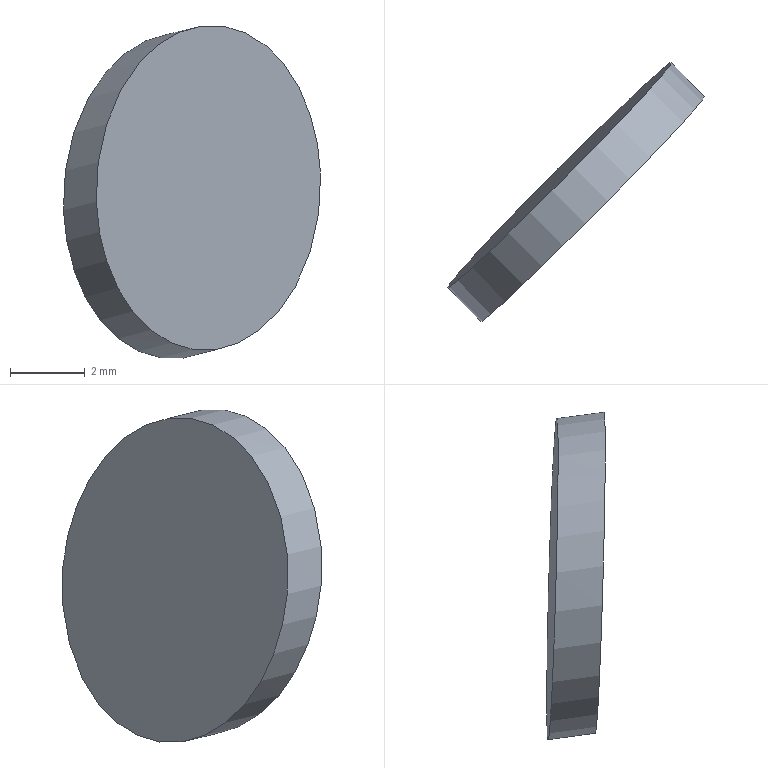Part | STEP file | gslz 2016.10.28-13_id1062_x_t | 1 solid | 3 faces | box 6.872 x 6.937 x 8.903 mm | volume 72.493 mm3 | spline 2 | cylinder 1 | commonest cylinder face diameters 8.5 x1
STEP:
#1=CARTESIAN_POINT('',(0.,0.,0.));
#2=DIRECTION('',(0.,0.,1.));
#3=DIRECTION('',(1.,0.,0.));
#4=AXIS2_PLACEMENT_3D('',#1,#2,#3);
#5=CARTESIAN_POINT('',(99.595,227.749,-30.31));
#6=VERTEX_POINT('',#5);
#7=CARTESIAN_POINT('',(93.608,221.761,-31.051));
#8=VERTEX_POINT('',#7);
#9=CARTESIAN_POINT('',(99.595,227.749,-30.31));
#10=CARTESIAN_POINT('',(99.637,227.846,-31.43));
#11=CARTESIAN_POINT('',(99.364,227.628,-32.586));
#12=CARTESIAN_POINT('',(98.322,226.666,-34.332));
#13=CARTESIAN_POINT('',(97.554,225.922,-34.908));
#14=CARTESIAN_POINT('',(95.969,224.337,-35.104));
#15=CARTESIAN_POINT('',(95.167,223.511,-34.722));
#16=CARTESIAN_POINT('',(94.005,222.269,-33.249));
#17=CARTESIAN_POINT('',(93.649,221.858,-32.171));
#18=CARTESIAN_POINT('',(93.608,221.761,-31.051));
#19=B_SPLINE_CURVE_WITH_KNOTS('',3,(#9,#10,#11,#12,#13,#14,#15,#16,#17,#18),.UNSPECIFIED.,.F.,.F.,(4,2,2,2,4),(0.,0.25,0.5,0.75,1.),.UNSPECIFIED.);
#20=CARTESIAN_POINT('',(82.862,211.656,-45.368));
#21=CARTESIAN_POINT('',(82.657,211.178,-39.851));
#22=CARTESIAN_POINT('',(82.452,210.7,-34.333));
#23=CARTESIAN_POINT('',(82.248,210.222,-28.816));
#24=CARTESIAN_POINT('',(82.043,209.744,-23.299));
#25=CARTESIAN_POINT('',(81.839,209.265,-17.782));
#26=CARTESIAN_POINT('',(88.082,216.876,-44.722));
#27=CARTESIAN_POINT('',(87.877,216.398,-39.205));
#28=CARTESIAN_POINT('',(87.673,215.92,-33.688));
#29=CARTESIAN_POINT('',(87.468,215.442,-28.17));
#30=CARTESIAN_POINT('',(87.264,214.964,-22.653));
#31=CARTESIAN_POINT('',(87.059,214.486,-17.136));
#32=CARTESIAN_POINT('',(93.302,222.096,-44.076));
#33=CARTESIAN_POINT('',(93.098,221.618,-38.559));
#34=CARTESIAN_POINT('',(92.893,221.14,-33.042));
#35=CARTESIAN_POINT('',(92.688,220.662,-27.524));
#36=CARTESIAN_POINT('',(92.484,220.184,-22.007));
#37=CARTESIAN_POINT('',(92.279,219.706,-16.49));
#38=CARTESIAN_POINT('',(98.522,227.317,-43.43));
#39=CARTESIAN_POINT('',(98.318,226.839,-37.913));
#40=CARTESIAN_POINT('',(98.113,226.361,-32.396));
#41=CARTESIAN_POINT('',(97.909,225.882,-26.879));
#42=CARTESIAN_POINT('',(97.704,225.404,-21.361));
#43=CARTESIAN_POINT('',(97.5,224.926,-15.844));
#44=CARTESIAN_POINT('',(103.743,232.537,-42.784));
#45=CARTESIAN_POINT('',(103.538,232.059,-37.267));
#46=CARTESIAN_POINT('',(103.334,231.581,-31.75));
#47=CARTESIAN_POINT('',(103.129,231.103,-26.233));
#48=CARTESIAN_POINT('',(102.924,230.625,-20.715));
#49=CARTESIAN_POINT('',(102.72,230.147,-15.198));
#50=CARTESIAN_POINT('',(108.963,237.757,-42.139));
#51=CARTESIAN_POINT('',(108.758,237.279,-36.621));
#52=CARTESIAN_POINT('',(108.554,236.801,-31.104));
#53=CARTESIAN_POINT('',(108.349,236.323,-25.587));
#54=CARTESIAN_POINT('',(108.145,235.845,-20.07));
#55=CARTESIAN_POINT('',(107.94,235.367,-14.552));
#56=B_SPLINE_SURFACE_WITH_KNOTS('',5,5,((#20,#21,#22,#23,#24,#25),(#26,#27,#28,#29,#30,#31),(#32,#33,#34,#35,#36,#37),(#38,#39,#40,#41,#42,#43),(#44,#45,#46,#47,#48,#49),(#50,#51,#52,#53,#54,#55)),.UNSPECIFIED.,.F.,.F.,.F.,(6,6),(6,6),(0.,1.),(0.,1.),.PIECEWISE_BEZIER_KNOTS.);
#57=CARTESIAN_POINT('',(0.6595,0.4687));
#58=CARTESIAN_POINT('',(0.6595,0.4613));
#59=CARTESIAN_POINT('',(0.6587,0.4465));
#60=CARTESIAN_POINT('',(0.6552,0.4248));
#61=CARTESIAN_POINT('',(0.6496,0.4039));
#62=CARTESIAN_POINT('',(0.6418,0.3843));
#63=CARTESIAN_POINT('',(0.6322,0.3663));
#64=CARTESIAN_POINT('',(0.6206,0.3503));
#65=CARTESIAN_POINT('',(0.6074,0.3368));
#66=CARTESIAN_POINT('',(0.593,0.326));
#67=CARTESIAN_POINT('',(0.5775,0.318));
#68=CARTESIAN_POINT('',(0.5613,0.313));
#69=CARTESIAN_POINT('',(0.5448,0.3113));
#70=CARTESIAN_POINT('',(0.5282,0.313));
#71=CARTESIAN_POINT('',(0.5121,0.318));
#72=CARTESIAN_POINT('',(0.4966,0.326));
#73=CARTESIAN_POINT('',(0.4821,0.3368));
#74=CARTESIAN_POINT('',(0.4689,0.3503));
#75=CARTESIAN_POINT('',(0.4574,0.3663));
#76=CARTESIAN_POINT('',(0.4477,0.3843));
#77=CARTESIAN_POINT('',(0.44,0.4039));
#78=CARTESIAN_POINT('',(0.4343,0.4248));
#79=CARTESIAN_POINT('',(0.4309,0.4465));
#80=CARTESIAN_POINT('',(0.4301,0.4613));
#81=CARTESIAN_POINT('',(0.4301,0.4687));
#82=B_SPLINE_CURVE_WITH_KNOTS('',3,(#57,#58,#59,#60,#61,#62,#63,#64,#65,#66,#67,#68,#69,#70,#71,#72,#73,#74,#75,#76,#77,#78,#79,#80,#81),.UNSPECIFIED.,.F.,.F.,(4,1,1,1,1,1,1,1,1,1,1,1,1,1,1,1,1,1,1,1,1,1,4),(0.,0.04545,0.09091,0.1364,0.1818,0.2273,0.2727,0.3182,0.3636,0.4091,0.4545,0.5,0.5455,0.5909,0.6364,0.6818,0.7273,0.7727,0.8182,0.8636,0.9091,0.9545,1.),.QUASI_UNIFORM_KNOTS.);
#83=(GEOMETRIC_REPRESENTATION_CONTEXT(2)PARAMETRIC_REPRESENTATION_CONTEXT()REPRESENTATION_CONTEXT('',''));
#84=DEFINITIONAL_REPRESENTATION('',(#82),#83);
#85=PCURVE('',#56,#84);
#86=CARTESIAN_POINT('',(96.602,224.755,-30.68));
#87=DIRECTION('',(0.6857,-0.7071,0.173));
#88=DIRECTION('',(-0.1835,0.06209,0.9811));
#89=AXIS2_PLACEMENT_3D('',#86,#87,#88);
#90=CYLINDRICAL_SURFACE('',#89,4.25);
#91=CARTESIAN_POINT('',(4.712,0.));
#92=CARTESIAN_POINT('',(4.665,-0.04253));
#93=CARTESIAN_POINT('',(4.571,-0.1275));
#94=CARTESIAN_POINT('',(4.43,-0.2526));
#95=CARTESIAN_POINT('',(4.288,-0.3729));
#96=CARTESIAN_POINT('',(4.146,-0.486));
#97=CARTESIAN_POINT('',(4.004,-0.5898));
#98=CARTESIAN_POINT('',(3.861,-0.6818));
#99=CARTESIAN_POINT('',(3.718,-0.7595));
#100=CARTESIAN_POINT('',(3.574,-0.822));
#101=CARTESIAN_POINT('',(3.43,-0.8682));
#102=CARTESIAN_POINT('',(3.286,-0.8968));
#103=CARTESIAN_POINT('',(3.142,-0.9067));
#104=CARTESIAN_POINT('',(2.997,-0.8968));
#105=CARTESIAN_POINT('',(2.853,-0.8682));
#106=CARTESIAN_POINT('',(2.709,-0.822));
#107=CARTESIAN_POINT('',(2.565,-0.7595));
#108=CARTESIAN_POINT('',(2.422,-0.6818));
#109=CARTESIAN_POINT('',(2.279,-0.5898));
#110=CARTESIAN_POINT('',(2.137,-0.486));
#111=CARTESIAN_POINT('',(1.995,-0.3729));
#112=CARTESIAN_POINT('',(1.853,-0.2526));
#113=CARTESIAN_POINT('',(1.712,-0.1275));
#114=CARTESIAN_POINT('',(1.618,-0.04253));
#115=CARTESIAN_POINT('',(1.571,0.));
#116=B_SPLINE_CURVE_WITH_KNOTS('',3,(#91,#92,#93,#94,#95,#96,#97,#98,#99,#100,#101,#102,#103,#104,#105,#106,#107,#108,#109,#110,#111,#112,#113,#114,#115),.UNSPECIFIED.,.F.,.F.,(4,1,1,1,1,1,1,1,1,1,1,1,1,1,1,1,1,1,1,1,1,1,4),(0.,0.04545,0.09091,0.1364,0.1818,0.2273,0.2727,0.3182,0.3636,0.4091,0.4545,0.5,0.5455,0.5909,0.6364,0.6818,0.7273,0.7727,0.8182,0.8636,0.9091,0.9545,1.),.QUASI_UNIFORM_KNOTS.);
#117=(GEOMETRIC_REPRESENTATION_CONTEXT(2)PARAMETRIC_REPRESENTATION_CONTEXT()REPRESENTATION_CONTEXT('',''));
#118=DEFINITIONAL_REPRESENTATION('',(#116),#117);
#119=PCURVE('',#90,#118);
#120=SURFACE_CURVE('',#19,(#85,#119),.PCURVE_S1.);
#121=EDGE_CURVE('',#6,#8,#120,.T.);
#122=ORIENTED_EDGE('',*,*,#121,.F.);
#123=CARTESIAN_POINT('',(93.608,221.761,-31.051));
#124=CARTESIAN_POINT('',(93.566,221.664,-29.931));
#125=CARTESIAN_POINT('',(93.839,221.881,-28.775));
#126=CARTESIAN_POINT('',(94.881,222.844,-27.029));
#127=CARTESIAN_POINT('',(95.649,223.588,-26.453));
#128=CARTESIAN_POINT('',(97.234,225.173,-26.256));
#129=CARTESIAN_POINT('',(98.036,225.999,-26.638));
#130=CARTESIAN_POINT('',(99.198,227.241,-28.112));
#131=CARTESIAN_POINT('',(99.554,227.652,-29.19));
#132=CARTESIAN_POINT('',(99.595,227.749,-30.31));
#133=B_SPLINE_CURVE_WITH_KNOTS('',3,(#123,#124,#125,#126,#127,#128,#129,#130,#131,#132),.UNSPECIFIED.,.F.,.F.,(4,2,2,2,4),(0.,0.25,0.5,0.75,1.),.UNSPECIFIED.);
#134=CARTESIAN_POINT('',(0.4301,0.4687));
#135=CARTESIAN_POINT('',(0.4301,0.476));
#136=CARTESIAN_POINT('',(0.4309,0.4908));
#137=CARTESIAN_POINT('',(0.4343,0.5125));
#138=CARTESIAN_POINT('',(0.44,0.5334));
#139=CARTESIAN_POINT('',(0.4477,0.553));
#140=CARTESIAN_POINT('',(0.4574,0.571));
#141=CARTESIAN_POINT('',(0.4689,0.587));
#142=CARTESIAN_POINT('',(0.4821,0.6005));
#143=CARTESIAN_POINT('',(0.4966,0.6113));
#144=CARTESIAN_POINT('',(0.5121,0.6193));
#145=CARTESIAN_POINT('',(0.5282,0.6243));
#146=CARTESIAN_POINT('',(0.5448,0.626));
#147=CARTESIAN_POINT('',(0.5613,0.6243));
#148=CARTESIAN_POINT('',(0.5775,0.6193));
#149=CARTESIAN_POINT('',(0.593,0.6113));
#150=CARTESIAN_POINT('',(0.6074,0.6005));
#151=CARTESIAN_POINT('',(0.6206,0.587));
#152=CARTESIAN_POINT('',(0.6322,0.571));
#153=CARTESIAN_POINT('',(0.6418,0.553));
#154=CARTESIAN_POINT('',(0.6496,0.5334));
#155=CARTESIAN_POINT('',(0.6552,0.5125));
#156=CARTESIAN_POINT('',(0.6587,0.4908));
#157=CARTESIAN_POINT('',(0.6595,0.476));
#158=CARTESIAN_POINT('',(0.6595,0.4687));
#159=B_SPLINE_CURVE_WITH_KNOTS('',3,(#134,#135,#136,#137,#138,#139,#140,#141,#142,#143,#144,#145,#146,#147,#148,#149,#150,#151,#152,#153,#154,#155,#156,#157,#158),.UNSPECIFIED.,.F.,.F.,(4,1,1,1,1,1,1,1,1,1,1,1,1,1,1,1,1,1,1,1,1,1,4),(0.,0.04545,0.09091,0.1364,0.1818,0.2273,0.2727,0.3182,0.3636,0.4091,0.4545,0.5,0.5455,0.5909,0.6364,0.6818,0.7273,0.7727,0.8182,0.8636,0.9091,0.9545,1.),.QUASI_UNIFORM_KNOTS.);
#160=(GEOMETRIC_REPRESENTATION_CONTEXT(2)PARAMETRIC_REPRESENTATION_CONTEXT()REPRESENTATION_CONTEXT('',''));
#161=DEFINITIONAL_REPRESENTATION('',(#159),#160);
#162=PCURVE('',#56,#161);
#163=CARTESIAN_POINT('',(7.854,0.));
#164=CARTESIAN_POINT('',(7.807,0.04253));
#165=CARTESIAN_POINT('',(7.713,0.1275));
#166=CARTESIAN_POINT('',(7.571,0.2526));
#167=CARTESIAN_POINT('',(7.43,0.3729));
#168=CARTESIAN_POINT('',(7.288,0.486));
#169=CARTESIAN_POINT('',(7.145,0.5898));
#170=CARTESIAN_POINT('',(7.003,0.6818));
#171=CARTESIAN_POINT('',(6.86,0.7595));
#172=CARTESIAN_POINT('',(6.716,0.822));
#173=CARTESIAN_POINT('',(6.572,0.8682));
#174=CARTESIAN_POINT('',(6.427,0.8968));
#175=CARTESIAN_POINT('',(6.283,0.9067));
#176=CARTESIAN_POINT('',(6.139,0.8968));
#177=CARTESIAN_POINT('',(5.995,0.8682));
#178=CARTESIAN_POINT('',(5.851,0.822));
#179=CARTESIAN_POINT('',(5.707,0.7595));
#180=CARTESIAN_POINT('',(5.564,0.6818));
#181=CARTESIAN_POINT('',(5.421,0.5898));
#182=CARTESIAN_POINT('',(5.279,0.486));
#183=CARTESIAN_POINT('',(5.137,0.3729));
#184=CARTESIAN_POINT('',(4.995,0.2526));
#185=CARTESIAN_POINT('',(4.854,0.1275));
#186=CARTESIAN_POINT('',(4.759,0.04253));
#187=CARTESIAN_POINT('',(4.712,0.));
#188=B_SPLINE_CURVE_WITH_KNOTS('',3,(#163,#164,#165,#166,#167,#168,#169,#170,#171,#172,#173,#174,#175,#176,#177,#178,#179,#180,#181,#182,#183,#184,#185,#186,#187),.UNSPECIFIED.,.F.,.F.,(4,1,1,1,1,1,1,1,1,1,1,1,1,1,1,1,1,1,1,1,1,1,4),(0.,0.04545,0.09091,0.1364,0.1818,0.2273,0.2727,0.3182,0.3636,0.4091,0.4545,0.5,0.5455,0.5909,0.6364,0.6818,0.7273,0.7727,0.8182,0.8636,0.9091,0.9545,1.),.QUASI_UNIFORM_KNOTS.);
#189=(GEOMETRIC_REPRESENTATION_CONTEXT(2)PARAMETRIC_REPRESENTATION_CONTEXT()REPRESENTATION_CONTEXT('',''));
#190=DEFINITIONAL_REPRESENTATION('',(#188),#189);
#191=PCURVE('',#90,#190);
#192=SURFACE_CURVE('',#133,(#162,#191),.PCURVE_S1.);
#193=EDGE_CURVE('',#8,#6,#192,.T.);
#194=ORIENTED_EDGE('',*,*,#193,.F.);
#195=EDGE_LOOP('',(#122,#194));
#196=FACE_BOUND('',#195,.F.);
#197=ADVANCED_FACE('',(#196),#56,.F.);
#198=ORIENTED_EDGE('',*,*,#193,.F.);
#199=CARTESIAN_POINT('',(94.484,220.858,-30.83));
#200=VERTEX_POINT('',#199);
#201=CARTESIAN_POINT('',(93.608,221.761,-31.051));
#202=CARTESIAN_POINT('',(94.484,220.858,-30.83));
#203=B_SPLINE_CURVE_WITH_KNOTS('',1,(#201,#202),.UNSPECIFIED.,.F.,.F.,(2,2),(0.,1.278),.PIECEWISE_BEZIER_KNOTS.);
#204=CARTESIAN_POINT('',(7.854,0.));
#205=DIRECTION('',(0.,1.));
#206=VECTOR('',#205,1.);
#207=LINE('',#204,#206);
#208=(GEOMETRIC_REPRESENTATION_CONTEXT(2)PARAMETRIC_REPRESENTATION_CONTEXT()REPRESENTATION_CONTEXT('',''));
#209=DEFINITIONAL_REPRESENTATION('',(#207),#208);
#210=PCURVE('',#90,#209);
#211=CARTESIAN_POINT('',(1.571,0.));
#212=DIRECTION('',(0.,1.));
#213=VECTOR('',#212,1.);
#214=LINE('',#211,#213);
#215=(GEOMETRIC_REPRESENTATION_CONTEXT(2)PARAMETRIC_REPRESENTATION_CONTEXT()REPRESENTATION_CONTEXT('',''));
#216=DEFINITIONAL_REPRESENTATION('',(#214),#215);
#217=PCURVE('',#90,#216);
#218=SEAM_CURVE('',#203,(#210,#217),.PCURVE_S1.);
#219=EDGE_CURVE('',#8,#200,#218,.T.);
#220=ORIENTED_EDGE('',*,*,#219,.T.);
#221=CARTESIAN_POINT('',(100.472,226.845,-30.089));
#222=VERTEX_POINT('',#221);
#223=CARTESIAN_POINT('',(94.484,220.858,-30.83));
#224=CARTESIAN_POINT('',(94.442,220.76,-29.707));
#225=CARTESIAN_POINT('',(94.714,220.977,-28.556));
#226=CARTESIAN_POINT('',(95.759,221.942,-26.805));
#227=CARTESIAN_POINT('',(96.525,222.684,-26.232));
#228=CARTESIAN_POINT('',(98.107,224.266,-26.035));
#229=CARTESIAN_POINT('',(98.908,225.091,-26.412));
#230=CARTESIAN_POINT('',(100.078,226.341,-27.895));
#231=CARTESIAN_POINT('',(100.43,226.748,-28.971));
#232=CARTESIAN_POINT('',(100.472,226.845,-30.089));
#233=B_SPLINE_CURVE_WITH_KNOTS('',3,(#223,#224,#225,#226,#227,#228,#229,#230,#231,#232),.UNSPECIFIED.,.F.,.F.,(4,2,2,2,4),(0.,0.25,0.5,0.75,1.),.UNSPECIFIED.);
#234=CARTESIAN_POINT('',(7.854,1.278));
#235=CARTESIAN_POINT('',(7.807,1.321));
#236=CARTESIAN_POINT('',(7.713,1.406));
#237=CARTESIAN_POINT('',(7.571,1.531));
#238=CARTESIAN_POINT('',(7.43,1.651));
#239=CARTESIAN_POINT('',(7.288,1.764));
#240=CARTESIAN_POINT('',(7.146,1.868));
#241=CARTESIAN_POINT('',(7.003,1.96));
#242=CARTESIAN_POINT('',(6.859,2.038));
#243=CARTESIAN_POINT('',(6.715,2.1));
#244=CARTESIAN_POINT('',(6.571,2.146));
#245=CARTESIAN_POINT('',(6.428,2.175));
#246=CARTESIAN_POINT('',(6.284,2.185));
#247=CARTESIAN_POINT('',(6.14,2.175));
#248=CARTESIAN_POINT('',(5.996,2.146));
#249=CARTESIAN_POINT('',(5.852,2.101));
#250=CARTESIAN_POINT('',(5.708,2.038));
#251=CARTESIAN_POINT('',(5.564,1.96));
#252=CARTESIAN_POINT('',(5.421,1.868));
#253=CARTESIAN_POINT('',(5.278,1.764));
#254=CARTESIAN_POINT('',(5.136,1.65));
#255=CARTESIAN_POINT('',(4.994,1.53));
#256=CARTESIAN_POINT('',(4.853,1.405));
#257=CARTESIAN_POINT('',(4.759,1.32));
#258=CARTESIAN_POINT('',(4.712,1.278));
#259=B_SPLINE_CURVE_WITH_KNOTS('',3,(#234,#235,#236,#237,#238,#239,#240,#241,#242,#243,#244,#245,#246,#247,#248,#249,#250,#251,#252,#253,#254,#255,#256,#257,#258),.UNSPECIFIED.,.F.,.F.,(4,1,1,1,1,1,1,1,1,1,1,1,1,1,1,1,1,1,1,1,1,1,4),(0.,0.04545,0.09091,0.1364,0.1818,0.2273,0.2727,0.3182,0.3636,0.4091,0.4545,0.5,0.5455,0.5909,0.6364,0.6818,0.7273,0.7727,0.8182,0.8636,0.9091,0.9545,1.),.QUASI_UNIFORM_KNOTS.);
#260=(GEOMETRIC_REPRESENTATION_CONTEXT(2)PARAMETRIC_REPRESENTATION_CONTEXT()REPRESENTATION_CONTEXT('',''));
#261=DEFINITIONAL_REPRESENTATION('',(#259),#260);
#262=PCURVE('',#90,#261);
#263=CARTESIAN_POINT('',(94.611,221.202,-35.228));
#264=CARTESIAN_POINT('',(94.502,220.949,-32.299));
#265=CARTESIAN_POINT('',(94.394,220.695,-29.369));
#266=CARTESIAN_POINT('',(94.285,220.441,-26.44));
#267=CARTESIAN_POINT('',(96.631,223.222,-34.978));
#268=CARTESIAN_POINT('',(96.522,222.968,-32.049));
#269=CARTESIAN_POINT('',(96.414,222.715,-29.12));
#270=CARTESIAN_POINT('',(96.305,222.461,-26.19));
#271=CARTESIAN_POINT('',(98.651,225.242,-34.728));
#272=CARTESIAN_POINT('',(98.542,224.988,-31.799));
#273=CARTESIAN_POINT('',(98.433,224.734,-28.87));
#274=CARTESIAN_POINT('',(98.325,224.48,-25.94));
#275=CARTESIAN_POINT('',(100.67,227.262,-34.478));
#276=CARTESIAN_POINT('',(100.562,227.008,-31.549));
#277=CARTESIAN_POINT('',(100.453,226.754,-28.62));
#278=CARTESIAN_POINT('',(100.345,226.5,-25.69));
#279=B_SPLINE_SURFACE_WITH_KNOTS('',3,3,((#263,#264,#265,#266),(#267,#268,#269,#270),(#271,#272,#273,#274),(#275,#276,#277,#278)),.UNSPECIFIED.,.F.,.F.,.F.,(4,4),(4,4),(0.,1.),(0.,1.),.PIECEWISE_BEZIER_KNOTS.);
#280=CARTESIAN_POINT('',(0.005929,0.5));
#281=CARTESIAN_POINT('',(0.005929,0.5232));
#282=CARTESIAN_POINT('',(0.00934,0.5696));
#283=CARTESIAN_POINT('',(0.02426,0.6377));
#284=CARTESIAN_POINT('',(0.04854,0.7032));
#285=CARTESIAN_POINT('',(0.08177,0.7648));
#286=CARTESIAN_POINT('',(0.1235,0.8213));
#287=CARTESIAN_POINT('',(0.1733,0.8716));
#288=CARTESIAN_POINT('',(0.2302,0.9139));
#289=CARTESIAN_POINT('',(0.2925,0.948));
#290=CARTESIAN_POINT('',(0.3592,0.9731));
#291=CARTESIAN_POINT('',(0.4287,0.9886));
#292=CARTESIAN_POINT('',(0.4998,0.994));
#293=CARTESIAN_POINT('',(0.5709,0.9887));
#294=CARTESIAN_POINT('',(0.6404,0.9732));
#295=CARTESIAN_POINT('',(0.7071,0.9482));
#296=CARTESIAN_POINT('',(0.7695,0.9142));
#297=CARTESIAN_POINT('',(0.8264,0.8717));
#298=CARTESIAN_POINT('',(0.8765,0.8213));
#299=CARTESIAN_POINT('',(0.9183,0.7646));
#300=CARTESIAN_POINT('',(0.9516,0.7029));
#301=CARTESIAN_POINT('',(0.9758,0.6374));
#302=CARTESIAN_POINT('',(0.9907,0.5694));
#303=CARTESIAN_POINT('',(0.9941,0.5231));
#304=CARTESIAN_POINT('',(0.9941,0.5));
#305=B_SPLINE_CURVE_WITH_KNOTS('',3,(#280,#281,#282,#283,#284,#285,#286,#287,#288,#289,#290,#291,#292,#293,#294,#295,#296,#297,#298,#299,#300,#301,#302,#303,#304),.UNSPECIFIED.,.F.,.F.,(4,1,1,1,1,1,1,1,1,1,1,1,1,1,1,1,1,1,1,1,1,1,4),(0.,0.04545,0.09091,0.1364,0.1818,0.2273,0.2727,0.3182,0.3636,0.4091,0.4545,0.5,0.5455,0.5909,0.6364,0.6818,0.7273,0.7727,0.8182,0.8636,0.9091,0.9545,1.),.QUASI_UNIFORM_KNOTS.);
#306=(GEOMETRIC_REPRESENTATION_CONTEXT(2)PARAMETRIC_REPRESENTATION_CONTEXT()REPRESENTATION_CONTEXT('',''));
#307=DEFINITIONAL_REPRESENTATION('',(#305),#306);
#308=PCURVE('',#279,#307);
#309=SURFACE_CURVE('',#233,(#262,#308),.PCURVE_S1.);
#310=EDGE_CURVE('',#200,#222,#309,.T.);
#311=ORIENTED_EDGE('',*,*,#310,.T.);
#312=CARTESIAN_POINT('',(100.472,226.845,-30.089));
#313=CARTESIAN_POINT('',(100.513,226.942,-31.211));
#314=CARTESIAN_POINT('',(100.242,226.726,-32.362));
#315=CARTESIAN_POINT('',(99.196,225.761,-34.113));
#316=CARTESIAN_POINT('',(98.43,225.018,-34.687));
#317=CARTESIAN_POINT('',(96.848,223.436,-34.883));
#318=CARTESIAN_POINT('',(96.047,222.612,-34.507));
#319=CARTESIAN_POINT('',(94.878,221.362,-33.024));
#320=CARTESIAN_POINT('',(94.525,220.954,-31.947));
#321=CARTESIAN_POINT('',(94.484,220.858,-30.83));
#322=B_SPLINE_CURVE_WITH_KNOTS('',3,(#312,#313,#314,#315,#316,#317,#318,#319,#320,#321),.UNSPECIFIED.,.F.,.F.,(4,2,2,2,4),(0.,0.25,0.5,0.75,1.),.UNSPECIFIED.);
#323=CARTESIAN_POINT('',(4.712,1.278));
#324=CARTESIAN_POINT('',(4.665,1.235));
#325=CARTESIAN_POINT('',(4.571,1.15));
#326=CARTESIAN_POINT('',(4.43,1.025));
#327=CARTESIAN_POINT('',(4.288,0.9051));
#328=CARTESIAN_POINT('',(4.146,0.792));
#329=CARTESIAN_POINT('',(4.004,0.6883));
#330=CARTESIAN_POINT('',(3.861,0.596));
#331=CARTESIAN_POINT('',(3.718,0.5182));
#332=CARTESIAN_POINT('',(3.574,0.4557));
#333=CARTESIAN_POINT('',(3.43,0.4097));
#334=CARTESIAN_POINT('',(3.286,0.3812));
#335=CARTESIAN_POINT('',(3.142,0.3713));
#336=CARTESIAN_POINT('',(2.998,0.3811));
#337=CARTESIAN_POINT('',(2.854,0.4094));
#338=CARTESIAN_POINT('',(2.71,0.4553));
#339=CARTESIAN_POINT('',(2.566,0.5178));
#340=CARTESIAN_POINT('',(2.423,0.5957));
#341=CARTESIAN_POINT('',(2.279,0.6883));
#342=CARTESIAN_POINT('',(2.137,0.7923));
#343=CARTESIAN_POINT('',(1.994,0.9056));
#344=CARTESIAN_POINT('',(1.853,1.026));
#345=CARTESIAN_POINT('',(1.712,1.151));
#346=CARTESIAN_POINT('',(1.618,1.235));
#347=CARTESIAN_POINT('',(1.571,1.278));
#348=B_SPLINE_CURVE_WITH_KNOTS('',3,(#323,#324,#325,#326,#327,#328,#329,#330,#331,#332,#333,#334,#335,#336,#337,#338,#339,#340,#341,#342,#343,#344,#345,#346,#347),.UNSPECIFIED.,.F.,.F.,(4,1,1,1,1,1,1,1,1,1,1,1,1,1,1,1,1,1,1,1,1,1,4),(0.,0.04545,0.09091,0.1364,0.1818,0.2273,0.2727,0.3182,0.3636,0.4091,0.4545,0.5,0.5455,0.5909,0.6364,0.6818,0.7273,0.7727,0.8182,0.8636,0.9091,0.9545,1.),.QUASI_UNIFORM_KNOTS.);
#349=(GEOMETRIC_REPRESENTATION_CONTEXT(2)PARAMETRIC_REPRESENTATION_CONTEXT()REPRESENTATION_CONTEXT('',''));
#350=DEFINITIONAL_REPRESENTATION('',(#348),#349);
#351=PCURVE('',#90,#350);
#352=CARTESIAN_POINT('',(0.9941,0.5));
#353=CARTESIAN_POINT('',(0.9941,0.4768));
#354=CARTESIAN_POINT('',(0.9907,0.4304));
#355=CARTESIAN_POINT('',(0.9757,0.3623));
#356=CARTESIAN_POINT('',(0.9515,0.2968));
#357=CARTESIAN_POINT('',(0.9182,0.2352));
#358=CARTESIAN_POINT('',(0.8765,0.1787));
#359=CARTESIAN_POINT('',(0.8267,0.1284));
#360=CARTESIAN_POINT('',(0.7698,0.08606));
#361=CARTESIAN_POINT('',(0.7075,0.052));
#362=CARTESIAN_POINT('',(0.6408,0.02691));
#363=CARTESIAN_POINT('',(0.5713,0.01137));
#364=CARTESIAN_POINT('',(0.5002,0.005981));
#365=CARTESIAN_POINT('',(0.4291,0.0113));
#366=CARTESIAN_POINT('',(0.3596,0.02676));
#367=CARTESIAN_POINT('',(0.2929,0.05178));
#368=CARTESIAN_POINT('',(0.2305,0.08581));
#369=CARTESIAN_POINT('',(0.1736,0.1283));
#370=CARTESIAN_POINT('',(0.1235,0.1787));
#371=CARTESIAN_POINT('',(0.08168,0.2354));
#372=CARTESIAN_POINT('',(0.04844,0.2971));
#373=CARTESIAN_POINT('',(0.02419,0.3626));
#374=CARTESIAN_POINT('',(0.009322,0.4306));
#375=CARTESIAN_POINT('',(0.005929,0.4769));
#376=CARTESIAN_POINT('',(0.005929,0.5));
#377=B_SPLINE_CURVE_WITH_KNOTS('',3,(#352,#353,#354,#355,#356,#357,#358,#359,#360,#361,#362,#363,#364,#365,#366,#367,#368,#369,#370,#371,#372,#373,#374,#375,#376),.UNSPECIFIED.,.F.,.F.,(4,1,1,1,1,1,1,1,1,1,1,1,1,1,1,1,1,1,1,1,1,1,4),(0.,0.04545,0.09091,0.1364,0.1818,0.2273,0.2727,0.3182,0.3636,0.4091,0.4545,0.5,0.5455,0.5909,0.6364,0.6818,0.7273,0.7727,0.8182,0.8636,0.9091,0.9545,1.),.QUASI_UNIFORM_KNOTS.);
#378=(GEOMETRIC_REPRESENTATION_CONTEXT(2)PARAMETRIC_REPRESENTATION_CONTEXT()REPRESENTATION_CONTEXT('',''));
#379=DEFINITIONAL_REPRESENTATION('',(#377),#378);
#380=PCURVE('',#279,#379);
#381=SURFACE_CURVE('',#322,(#351,#380),.PCURVE_S1.);
#382=EDGE_CURVE('',#222,#200,#381,.T.);
#383=ORIENTED_EDGE('',*,*,#382,.T.);
#384=ORIENTED_EDGE('',*,*,#219,.F.);
#385=ORIENTED_EDGE('',*,*,#121,.F.);
#386=EDGE_LOOP('',(#198,#220,#311,#383,#384,#385));
#387=FACE_BOUND('',#386,.T.);
#388=ADVANCED_FACE('',(#387),#90,.T.);
#389=ORIENTED_EDGE('',*,*,#382,.F.);
#390=ORIENTED_EDGE('',*,*,#310,.F.);
#391=EDGE_LOOP('',(#389,#390));
#392=FACE_BOUND('',#391,.T.);
#393=ADVANCED_FACE('',(#392),#279,.T.);
#394=CLOSED_SHELL('',(#197,#388,#393));
#395=MANIFOLD_SOLID_BREP('',#394);
#396=(LENGTH_UNIT()NAMED_UNIT(*)SI_UNIT(.MILLI.,.METRE.));
#397=UNCERTAINTY_MEASURE_WITH_UNIT(LENGTH_MEASURE(0.005),#396,'','');
#398=(NAMED_UNIT(*)PLANE_ANGLE_UNIT()SI_UNIT($,.RADIAN.));
#399=(NAMED_UNIT(*)SI_UNIT($,.STERADIAN.)SOLID_ANGLE_UNIT());
#400=(GEOMETRIC_REPRESENTATION_CONTEXT(3)GLOBAL_UNCERTAINTY_ASSIGNED_CONTEXT((#397))GLOBAL_UNIT_ASSIGNED_CONTEXT((#396,#398,#399))REPRESENTATION_CONTEXT('',''));
#401=ADVANCED_BREP_SHAPE_REPRESENTATION('',(#4,#395),#400);